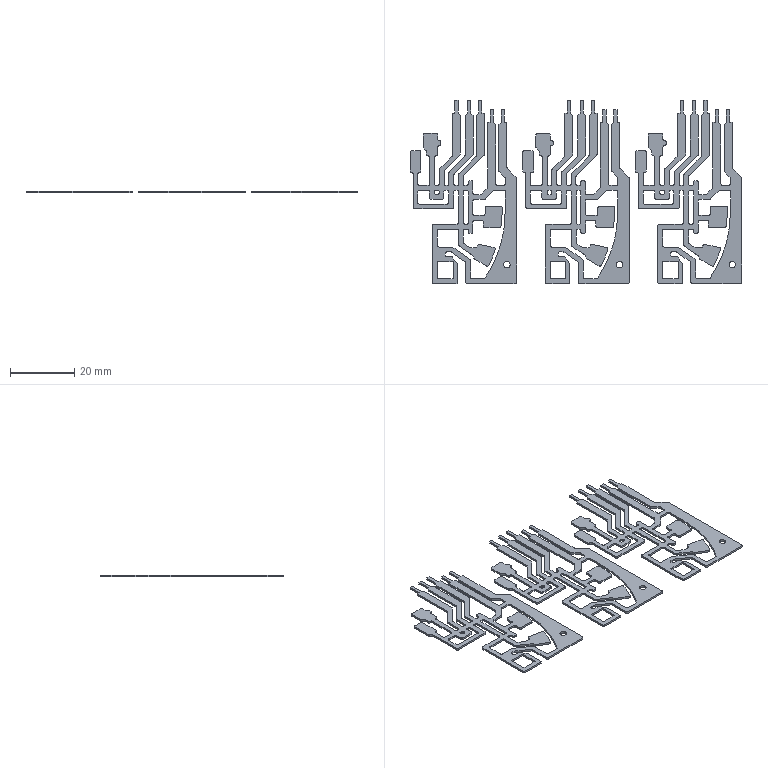Part | NX | features BREP 3 | 6 solids | 1602 faces | box 103.1 x 57.003 x 0.6 mm | volume 2955 mm3 | plane 876 | cylinder 726 | commonest cylinder face diameters 1 x690 2 x6 69.173 x6 72.496 x6 72.701 x6 163.294 x6